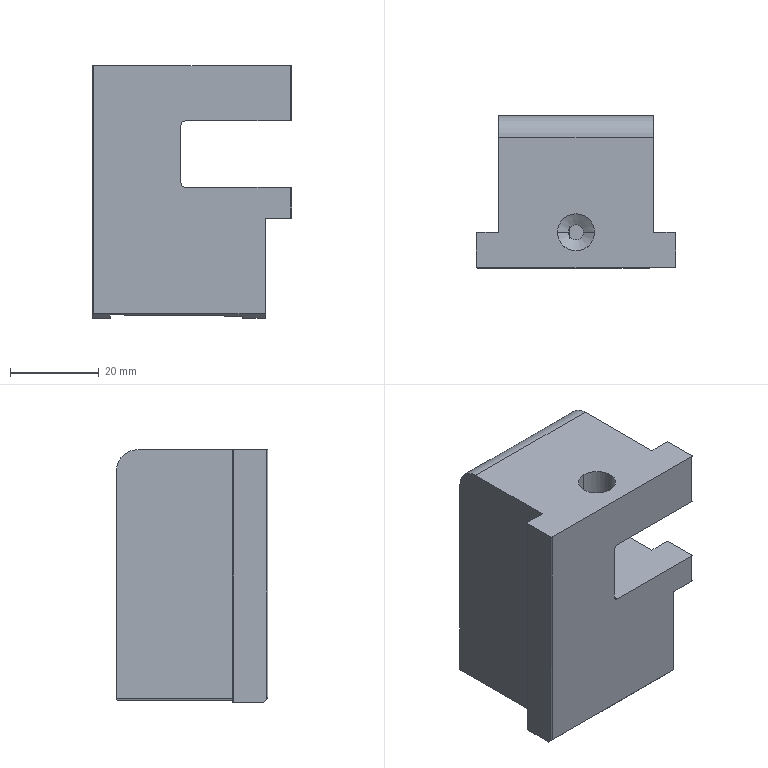Part | STEP file | dao nhan khuon dap 3m6 | 1 solid | 44 faces | box 45 x 34.3 x 57.1 mm | volume 58767 mm3 | plane 27 | cylinder 13 | cone 4 | commonest cylinder face diameters 0.6 x6 1 x2 2 x2 8.376 x2 10 x1